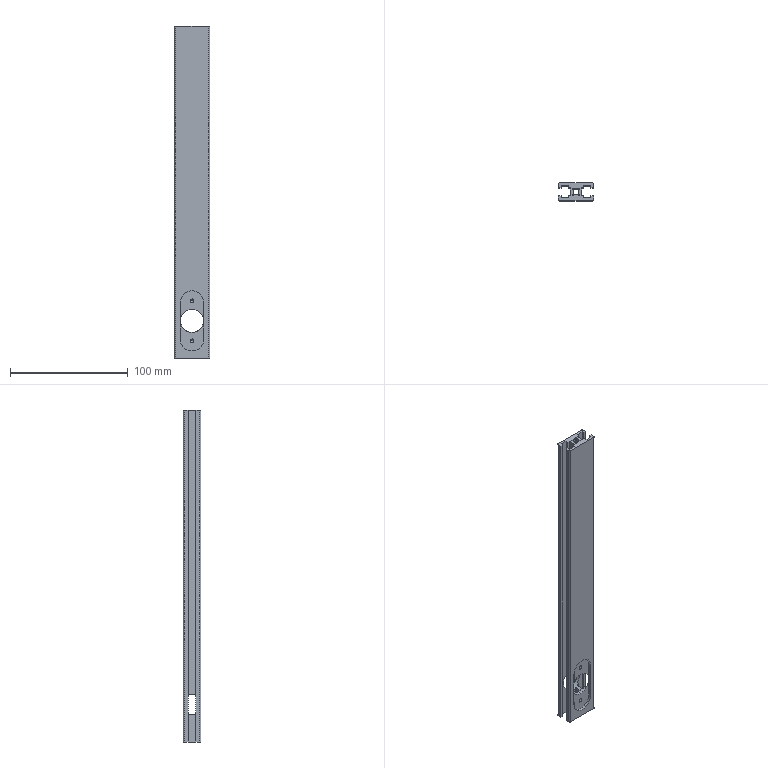Part | NX | features BREP 1 | 1 solid | 152 faces | box 30 x 15 x 282 mm | volume 63084 mm3 | plane 75 | cylinder 69 | cone 8 | commonest cylinder face diameters 1 x24 5 x24 3.3 x8 2 x4 6.8 x4 20 x3